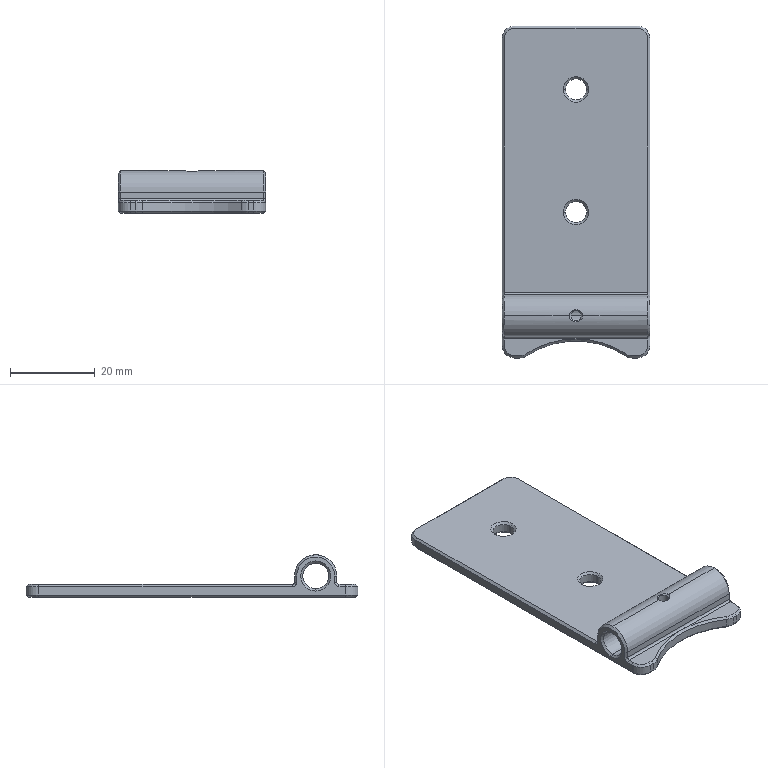Part | SolidWorks | features MoveFace 4, Fillet 2, 3DProfileFeature 1, Chamfer 1, Extrusion 1, HoleWzd 1, ICE 1 | 1 solid | 81 faces | box 34.9 x 78.5 x 10 mm | volume 8847 mm3 | cone 35 | plane 27 | cylinder 19 | commonest cylinder face diameters 6 x6 5 x4 1 x2 2.5 x2 6.1 x2 10 x2